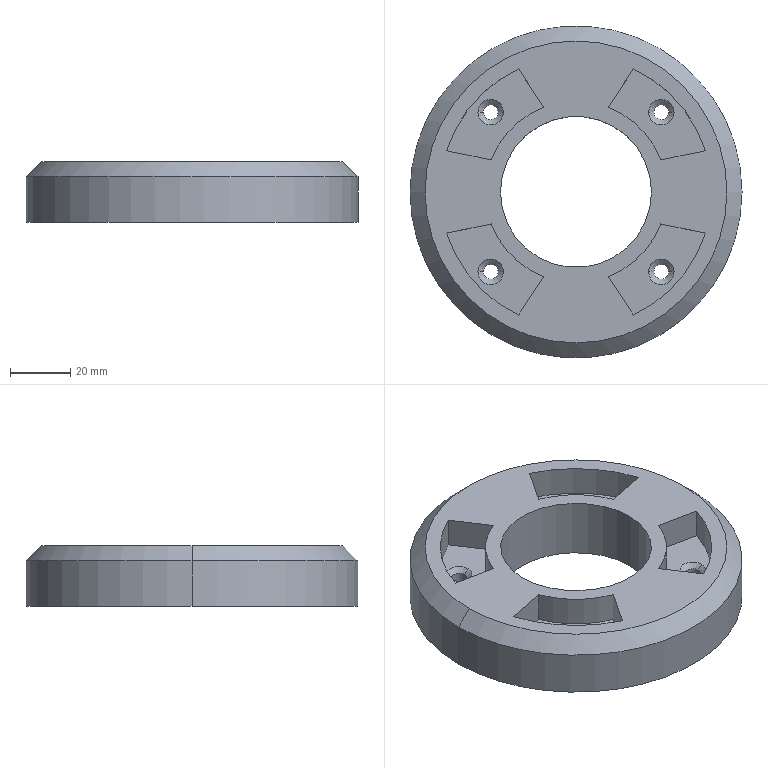Part | SolidWorks | features MirrorPattern 2, 3DProfileFeature 1, Chamfer 1, Extrusion 1, HoleWzd 1, ICE 1 | 1 solid | 44 faces | box 110 x 110 x 20 mm | volume 126964 mm3 | cylinder 20 | plane 14 | cone 10 | commonest cylinder face diameters 4.915 x8 60 x4 90 x4 50 x2 110 x2
STEP:
#1=CARTESIAN_POINT('',(25.827,-26.458,8.524));
#2=VERTEX_POINT('',#1);
#3=CARTESIAN_POINT('',(30.742,-26.458,8.524));
#4=VERTEX_POINT('',#3);
#5=CARTESIAN_POINT('',(28.284,-26.458,8.524));
#6=DIRECTION('',(0.,0.,1.));
#7=DIRECTION('',(1.,0.,0.));
#8=AXIS2_PLACEMENT_3D('',#5,#6,#7);
#9=CIRCLE('',#8,2.457);
#10=EDGE_CURVE('',#2,#4,#9,.T.);
#11=ORIENTED_EDGE('',*,*,#10,.F.);
#12=CARTESIAN_POINT('',(24.068,-26.458,10.));
#13=VERTEX_POINT('',#12);
#14=CARTESIAN_POINT('',(24.068,-26.458,10.));
#15=DIRECTION('',(-0.766,0.,0.6428));
#16=VECTOR('',#15,1000.);
#17=LINE('',#14,#16);
#18=EDGE_CURVE('',#2,#13,#17,.T.);
#19=ORIENTED_EDGE('',*,*,#18,.T.);
#20=CARTESIAN_POINT('',(32.501,-26.458,10.));
#21=VERTEX_POINT('',#20);
#22=CARTESIAN_POINT('',(28.284,-26.458,10.));
#23=DIRECTION('',(0.,0.,1.));
#24=DIRECTION('',(1.,0.,0.));
#25=AXIS2_PLACEMENT_3D('',#22,#23,#24);
#26=CIRCLE('',#25,4.216);
#27=EDGE_CURVE('',#13,#21,#26,.T.);
#28=ORIENTED_EDGE('',*,*,#27,.T.);
#29=CARTESIAN_POINT('',(32.501,-26.458,10.));
#30=DIRECTION('',(0.766,0.,0.6428));
#31=VECTOR('',#30,1000.);
#32=LINE('',#29,#31);
#33=EDGE_CURVE('',#4,#21,#32,.T.);
#34=ORIENTED_EDGE('',*,*,#33,.F.);
#35=EDGE_LOOP('',(#11,#19,#28,#34));
#36=FACE_OUTER_BOUND('',#35,.T.);
#37=CARTESIAN_POINT('',(28.284,-26.458,10.));
#38=DIRECTION('',(0.,0.,1.));
#39=DIRECTION('',(1.,0.,0.));
#40=AXIS2_PLACEMENT_3D('',#37,#38,#39);
#41=CONICAL_SURFACE('',#40,4.216,0.8727);
#42=ADVANCED_FACE('',(#36),#41,.F.);
#43=CARTESIAN_POINT('',(25.827,-26.458,0.));
#44=VERTEX_POINT('',#43);
#45=CARTESIAN_POINT('',(30.742,-26.458,0.));
#46=VERTEX_POINT('',#45);
#47=CARTESIAN_POINT('',(28.284,-26.458,0.));
#48=DIRECTION('',(0.,0.,1.));
#49=DIRECTION('',(1.,0.,0.));
#50=AXIS2_PLACEMENT_3D('',#47,#48,#49);
#51=CIRCLE('',#50,2.457);
#52=EDGE_CURVE('',#44,#46,#51,.T.);
#53=ORIENTED_EDGE('',*,*,#52,.F.);
#54=CARTESIAN_POINT('',(25.827,-26.458,10.));
#55=DIRECTION('',(0.,0.,1.));
#56=VECTOR('',#55,1000.);
#57=LINE('',#54,#56);
#58=EDGE_CURVE('',#44,#2,#57,.T.);
#59=ORIENTED_EDGE('',*,*,#58,.T.);
#60=ORIENTED_EDGE('',*,*,#10,.T.);
#61=CARTESIAN_POINT('',(30.742,-26.458,10.));
#62=DIRECTION('',(0.,0.,1.));
#63=VECTOR('',#62,1000.);
#64=LINE('',#61,#63);
#65=EDGE_CURVE('',#46,#4,#64,.T.);
#66=ORIENTED_EDGE('',*,*,#65,.F.);
#67=EDGE_LOOP('',(#53,#59,#60,#66));
#68=FACE_OUTER_BOUND('',#67,.T.);
#69=CARTESIAN_POINT('',(28.284,-26.458,10.));
#70=DIRECTION('',(0.,0.,1.));
#71=DIRECTION('',(1.,0.,0.));
#72=AXIS2_PLACEMENT_3D('',#69,#70,#71);
#73=CYLINDRICAL_SURFACE('',#72,2.457);
#74=ADVANCED_FACE('',(#68),#73,.F.);
#75=CARTESIAN_POINT('',(-30.742,-26.458,8.524));
#76=VERTEX_POINT('',#75);
#77=CARTESIAN_POINT('',(-25.827,-26.458,8.524));
#78=VERTEX_POINT('',#77);
#79=CARTESIAN_POINT('',(-28.284,-26.458,8.524));
#80=DIRECTION('',(0.,0.,1.));
#81=DIRECTION('',(1.,0.,0.));
#82=AXIS2_PLACEMENT_3D('',#79,#80,#81);
#83=CIRCLE('',#82,2.457);
#84=EDGE_CURVE('',#76,#78,#83,.T.);
#85=ORIENTED_EDGE('',*,*,#84,.F.);
#86=CARTESIAN_POINT('',(-32.501,-26.458,10.));
#87=VERTEX_POINT('',#86);
#88=CARTESIAN_POINT('',(-32.501,-26.458,10.));
#89=DIRECTION('',(-0.766,0.,0.6428));
#90=VECTOR('',#89,1000.);
#91=LINE('',#88,#90);
#92=EDGE_CURVE('',#76,#87,#91,.T.);
#93=ORIENTED_EDGE('',*,*,#92,.T.);
#94=CARTESIAN_POINT('',(-24.068,-26.458,10.));
#95=VERTEX_POINT('',#94);
#96=CARTESIAN_POINT('',(-28.284,-26.458,10.));
#97=DIRECTION('',(0.,0.,1.));
#98=DIRECTION('',(1.,0.,0.));
#99=AXIS2_PLACEMENT_3D('',#96,#97,#98);
#100=CIRCLE('',#99,4.216);
#101=EDGE_CURVE('',#87,#95,#100,.T.);
#102=ORIENTED_EDGE('',*,*,#101,.T.);
#103=CARTESIAN_POINT('',(-24.068,-26.458,10.));
#104=DIRECTION('',(0.766,0.,0.6428));
#105=VECTOR('',#104,1000.);
#106=LINE('',#103,#105);
#107=EDGE_CURVE('',#78,#95,#106,.T.);
#108=ORIENTED_EDGE('',*,*,#107,.F.);
#109=EDGE_LOOP('',(#85,#93,#102,#108));
#110=FACE_OUTER_BOUND('',#109,.T.);
#111=CARTESIAN_POINT('',(-28.284,-26.458,10.));
#112=DIRECTION('',(0.,0.,1.));
#113=DIRECTION('',(1.,0.,0.));
#114=AXIS2_PLACEMENT_3D('',#111,#112,#113);
#115=CONICAL_SURFACE('',#114,4.216,0.8727);
#116=ADVANCED_FACE('',(#110),#115,.F.);
#117=CARTESIAN_POINT('',(-30.742,-26.458,0.));
#118=VERTEX_POINT('',#117);
#119=CARTESIAN_POINT('',(-25.827,-26.458,0.));
#120=VERTEX_POINT('',#119);
#121=CARTESIAN_POINT('',(-28.284,-26.458,0.));
#122=DIRECTION('',(0.,0.,1.));
#123=DIRECTION('',(1.,0.,0.));
#124=AXIS2_PLACEMENT_3D('',#121,#122,#123);
#125=CIRCLE('',#124,2.457);
#126=EDGE_CURVE('',#118,#120,#125,.T.);
#127=ORIENTED_EDGE('',*,*,#126,.F.);
#128=CARTESIAN_POINT('',(-30.742,-26.458,10.));
#129=DIRECTION('',(0.,0.,1.));
#130=VECTOR('',#129,1000.);
#131=LINE('',#128,#130);
#132=EDGE_CURVE('',#118,#76,#131,.T.);
#133=ORIENTED_EDGE('',*,*,#132,.T.);
#134=ORIENTED_EDGE('',*,*,#84,.T.);
#135=CARTESIAN_POINT('',(-25.827,-26.458,10.));
#136=DIRECTION('',(0.,0.,1.));
#137=VECTOR('',#136,1000.);
#138=LINE('',#135,#137);
#139=EDGE_CURVE('',#120,#78,#138,.T.);
#140=ORIENTED_EDGE('',*,*,#139,.F.);
#141=EDGE_LOOP('',(#127,#133,#134,#140));
#142=FACE_OUTER_BOUND('',#141,.T.);
#143=CARTESIAN_POINT('',(-28.284,-26.458,10.));
#144=DIRECTION('',(0.,0.,1.));
#145=DIRECTION('',(1.,0.,0.));
#146=AXIS2_PLACEMENT_3D('',#143,#144,#145);
#147=CYLINDRICAL_SURFACE('',#146,2.457);
#148=ADVANCED_FACE('',(#142),#147,.F.);
#149=CARTESIAN_POINT('',(25.827,26.458,8.524));
#150=VERTEX_POINT('',#149);
#151=CARTESIAN_POINT('',(30.742,26.458,8.524));
#152=VERTEX_POINT('',#151);
#153=CARTESIAN_POINT('',(28.284,26.458,8.524));
#154=DIRECTION('',(0.,0.,1.));
#155=DIRECTION('',(1.,0.,0.));
#156=AXIS2_PLACEMENT_3D('',#153,#154,#155);
#157=CIRCLE('',#156,2.457);
#158=EDGE_CURVE('',#150,#152,#157,.T.);
#159=ORIENTED_EDGE('',*,*,#158,.F.);
#160=CARTESIAN_POINT('',(24.068,26.458,10.));
#161=VERTEX_POINT('',#160);
#162=CARTESIAN_POINT('',(24.068,26.458,10.));
#163=DIRECTION('',(-0.766,0.,0.6428));
#164=VECTOR('',#163,1000.);
#165=LINE('',#162,#164);
#166=EDGE_CURVE('',#150,#161,#165,.T.);
#167=ORIENTED_EDGE('',*,*,#166,.T.);
#168=CARTESIAN_POINT('',(32.501,26.458,10.));
#169=VERTEX_POINT('',#168);
#170=CARTESIAN_POINT('',(28.284,26.458,10.));
#171=DIRECTION('',(0.,0.,1.));
#172=DIRECTION('',(1.,0.,0.));
#173=AXIS2_PLACEMENT_3D('',#170,#171,#172);
#174=CIRCLE('',#173,4.216);
#175=EDGE_CURVE('',#161,#169,#174,.T.);
#176=ORIENTED_EDGE('',*,*,#175,.T.);
#177=CARTESIAN_POINT('',(32.501,26.458,10.));
#178=DIRECTION('',(0.766,0.,0.6428));
#179=VECTOR('',#178,1000.);
#180=LINE('',#177,#179);
#181=EDGE_CURVE('',#152,#169,#180,.T.);
#182=ORIENTED_EDGE('',*,*,#181,.F.);
#183=EDGE_LOOP('',(#159,#167,#176,#182));
#184=FACE_OUTER_BOUND('',#183,.T.);
#185=CARTESIAN_POINT('',(28.284,26.458,10.));
#186=DIRECTION('',(0.,0.,1.));
#187=DIRECTION('',(1.,0.,0.));
#188=AXIS2_PLACEMENT_3D('',#185,#186,#187);
#189=CONICAL_SURFACE('',#188,4.216,0.8727);
#190=ADVANCED_FACE('',(#184),#189,.F.);
#191=CARTESIAN_POINT('',(25.827,26.458,0.));
#192=VERTEX_POINT('',#191);
#193=CARTESIAN_POINT('',(30.742,26.458,0.));
#194=VERTEX_POINT('',#193);
#195=CARTESIAN_POINT('',(28.284,26.458,0.));
#196=DIRECTION('',(0.,0.,1.));
#197=DIRECTION('',(1.,0.,0.));
#198=AXIS2_PLACEMENT_3D('',#195,#196,#197);
#199=CIRCLE('',#198,2.457);
#200=EDGE_CURVE('',#192,#194,#199,.T.);
#201=ORIENTED_EDGE('',*,*,#200,.F.);
#202=CARTESIAN_POINT('',(25.827,26.458,10.));
#203=DIRECTION('',(0.,0.,1.));
#204=VECTOR('',#203,1000.);
#205=LINE('',#202,#204);
#206=EDGE_CURVE('',#192,#150,#205,.T.);
#207=ORIENTED_EDGE('',*,*,#206,.T.);
#208=ORIENTED_EDGE('',*,*,#158,.T.);
#209=CARTESIAN_POINT('',(30.742,26.458,10.));
#210=DIRECTION('',(0.,0.,1.));
#211=VECTOR('',#210,1000.);
#212=LINE('',#209,#211);
#213=EDGE_CURVE('',#194,#152,#212,.T.);
#214=ORIENTED_EDGE('',*,*,#213,.F.);
#215=EDGE_LOOP('',(#201,#207,#208,#214));
#216=FACE_OUTER_BOUND('',#215,.T.);
#217=CARTESIAN_POINT('',(28.284,26.458,10.));
#218=DIRECTION('',(0.,0.,1.));
#219=DIRECTION('',(1.,0.,0.));
#220=AXIS2_PLACEMENT_3D('',#217,#218,#219);
#221=CYLINDRICAL_SURFACE('',#220,2.457);
#222=ADVANCED_FACE('',(#216),#221,.F.);
#223=CARTESIAN_POINT('',(-30.742,26.458,8.524));
#224=VERTEX_POINT('',#223);
#225=CARTESIAN_POINT('',(-25.827,26.458,8.524));
#226=VERTEX_POINT('',#225);
#227=CARTESIAN_POINT('',(-28.284,26.458,8.524));
#228=DIRECTION('',(0.,0.,1.));
#229=DIRECTION('',(1.,0.,0.));
#230=AXIS2_PLACEMENT_3D('',#227,#228,#229);
#231=CIRCLE('',#230,2.457);
#232=EDGE_CURVE('',#224,#226,#231,.T.);
#233=ORIENTED_EDGE('',*,*,#232,.F.);
#234=CARTESIAN_POINT('',(-32.501,26.458,10.));
#235=VERTEX_POINT('',#234);
#236=CARTESIAN_POINT('',(-32.501,26.458,10.));
#237=DIRECTION('',(-0.766,0.,0.6428));
#238=VECTOR('',#237,1000.);
#239=LINE('',#236,#238);
#240=EDGE_CURVE('',#224,#235,#239,.T.);
#241=ORIENTED_EDGE('',*,*,#240,.T.);
#242=CARTESIAN_POINT('',(-24.068,26.458,10.));
#243=VERTEX_POINT('',#242);
#244=CARTESIAN_POINT('',(-28.284,26.458,10.));
#245=DIRECTION('',(0.,0.,1.));
#246=DIRECTION('',(1.,0.,0.));
#247=AXIS2_PLACEMENT_3D('',#244,#245,#246);
#248=CIRCLE('',#247,4.216);
#249=EDGE_CURVE('',#235,#243,#248,.T.);
#250=ORIENTED_EDGE('',*,*,#249,.T.);
#251=CARTESIAN_POINT('',(-24.068,26.458,10.));
#252=DIRECTION('',(0.766,0.,0.6428));
#253=VECTOR('',#252,1000.);
#254=LINE('',#251,#253);
#255=EDGE_CURVE('',#226,#243,#254,.T.);
#256=ORIENTED_EDGE('',*,*,#255,.F.);
#257=EDGE_LOOP('',(#233,#241,#250,#256));
#258=FACE_OUTER_BOUND('',#257,.T.);
#259=CARTESIAN_POINT('',(-28.284,26.458,10.));
#260=DIRECTION('',(0.,0.,1.));
#261=DIRECTION('',(1.,0.,0.));
#262=AXIS2_PLACEMENT_3D('',#259,#260,#261);
#263=CONICAL_SURFACE('',#262,4.216,0.8727);
#264=ADVANCED_FACE('',(#258),#263,.F.);
#265=CARTESIAN_POINT('',(-30.742,26.458,0.));
#266=VERTEX_POINT('',#265);
#267=CARTESIAN_POINT('',(-25.827,26.458,0.));
#268=VERTEX_POINT('',#267);
#269=CARTESIAN_POINT('',(-28.284,26.458,0.));
#270=DIRECTION('',(0.,0.,1.));
#271=DIRECTION('',(1.,0.,0.));
#272=AXIS2_PLACEMENT_3D('',#269,#270,#271);
#273=CIRCLE('',#272,2.457);
#274=EDGE_CURVE('',#266,#268,#273,.T.);
#275=ORIENTED_EDGE('',*,*,#274,.F.);
#276=CARTESIAN_POINT('',(-30.742,26.458,10.));
#277=DIRECTION('',(0.,0.,1.));
#278=VECTOR('',#277,1000.);
#279=LINE('',#276,#278);
#280=EDGE_CURVE('',#266,#224,#279,.T.);
#281=ORIENTED_EDGE('',*,*,#280,.T.);
#282=ORIENTED_EDGE('',*,*,#232,.T.);
#283=CARTESIAN_POINT('',(-25.827,26.458,10.));
#284=DIRECTION('',(0.,0.,1.));
#285=VECTOR('',#284,1000.);
#286=LINE('',#283,#285);
#287=EDGE_CURVE('',#268,#226,#286,.T.);
#288=ORIENTED_EDGE('',*,*,#287,.F.);
#289=EDGE_LOOP('',(#275,#281,#282,#288));
#290=FACE_OUTER_BOUND('',#289,.T.);
#291=CARTESIAN_POINT('',(-28.284,26.458,10.));
#292=DIRECTION('',(0.,0.,1.));
#293=DIRECTION('',(1.,0.,0.));
#294=AXIS2_PLACEMENT_3D('',#291,#292,#293);
#295=CYLINDRICAL_SURFACE('',#294,2.457);
#296=ADVANCED_FACE('',(#290),#295,.F.);
#297=CARTESIAN_POINT('',(50.,0.,20.));
#298=VERTEX_POINT('',#297);
#299=CARTESIAN_POINT('',(-50.,0.,20.));
#300=VERTEX_POINT('',#299);
#301=CARTESIAN_POINT('',(0.,0.,20.));
#302=DIRECTION('',(0.,0.,1.));
#303=DIRECTION('',(1.,0.,0.));
#304=AXIS2_PLACEMENT_3D('',#301,#302,#303);
#305=CIRCLE('',#304,50.);
#306=EDGE_CURVE('',#298,#300,#305,.T.);
#307=ORIENTED_EDGE('',*,*,#306,.F.);
#308=CARTESIAN_POINT('',(55.,0.,15.));
#309=VERTEX_POINT('',#308);
#310=CARTESIAN_POINT('',(50.,0.,20.));
#311=DIRECTION('',(0.7071,0.,-0.7071));
#312=VECTOR('',#311,1000.);
#313=LINE('',#310,#312);
#314=EDGE_CURVE('',#298,#309,#313,.T.);
#315=ORIENTED_EDGE('',*,*,#314,.T.);
#316=CARTESIAN_POINT('',(-55.,0.,15.));
#317=VERTEX_POINT('',#316);
#318=CARTESIAN_POINT('',(0.,0.,15.));
#319=DIRECTION('',(0.,0.,-1.));
#320=DIRECTION('',(1.,0.,0.));
#321=AXIS2_PLACEMENT_3D('',#318,#319,#320);
#322=CIRCLE('',#321,55.);
#323=EDGE_CURVE('',#317,#309,#322,.T.);
#324=ORIENTED_EDGE('',*,*,#323,.F.);
#325=CARTESIAN_POINT('',(-50.,0.,20.));
#326=DIRECTION('',(-0.7071,0.,-0.7071));
#327=VECTOR('',#326,1000.);
#328=LINE('',#325,#327);
#329=EDGE_CURVE('',#300,#317,#328,.T.);
#330=ORIENTED_EDGE('',*,*,#329,.F.);
#331=EDGE_LOOP('',(#307,#315,#324,#330));
#332=FACE_OUTER_BOUND('',#331,.T.);
#333=CARTESIAN_POINT('',(0.,0.,20.));
#334=DIRECTION('',(0.,0.,-1.));
#335=DIRECTION('',(-1.,0.,0.));
#336=AXIS2_PLACEMENT_3D('',#333,#334,#335);
#337=CONICAL_SURFACE('',#336,50.,0.7854);
#338=ADVANCED_FACE('',(#332),#337,.T.);
#339=CARTESIAN_POINT('',(-25.,0.,20.));
#340=VERTEX_POINT('',#339);
#341=CARTESIAN_POINT('',(25.,0.,20.));
#342=VERTEX_POINT('',#341);
#343=CARTESIAN_POINT('',(0.,0.,20.));
#344=DIRECTION('',(0.,0.,1.));
#345=DIRECTION('',(1.,0.,0.));
#346=AXIS2_PLACEMENT_3D('',#343,#344,#345);
#347=CIRCLE('',#346,25.);
#348=EDGE_CURVE('',#340,#342,#347,.T.);
#349=ORIENTED_EDGE('',*,*,#348,.T.);
#350=CARTESIAN_POINT('',(25.,0.,0.));
#351=VERTEX_POINT('',#350);
#352=CARTESIAN_POINT('',(25.,0.,20.));
#353=DIRECTION('',(0.,0.,-1.));
#354=VECTOR('',#353,1000.);
#355=LINE('',#352,#354);
#356=EDGE_CURVE('',#342,#351,#355,.T.);
#357=ORIENTED_EDGE('',*,*,#356,.T.);
#358=CARTESIAN_POINT('',(-25.,0.,0.));
#359=VERTEX_POINT('',#358);
#360=CARTESIAN_POINT('',(0.,0.,0.));
#361=DIRECTION('',(0.,0.,1.));
#362=DIRECTION('',(1.,0.,0.));
#363=AXIS2_PLACEMENT_3D('',#360,#361,#362);
#364=CIRCLE('',#363,25.);
#365=EDGE_CURVE('',#359,#351,#364,.T.);
#366=ORIENTED_EDGE('',*,*,#365,.F.);
#367=CARTESIAN_POINT('',(-25.,0.,20.));
#368=DIRECTION('',(0.,0.,-1.));
#369=VECTOR('',#368,1000.);
#370=LINE('',#367,#369);
#371=EDGE_CURVE('',#340,#359,#370,.T.);
#372=ORIENTED_EDGE('',*,*,#371,.F.);
#373=EDGE_LOOP('',(#349,#357,#366,#372));
#374=FACE_OUTER_BOUND('',#373,.T.);
#375=CARTESIAN_POINT('',(0.,0.,20.));
#376=DIRECTION('',(0.,0.,-1.));
#377=DIRECTION('',(-1.,0.,0.));
#378=AXIS2_PLACEMENT_3D('',#375,#376,#377);
#379=CYLINDRICAL_SURFACE('',#378,25.);
#380=ADVANCED_FACE('',(#374),#379,.F.);
#381=ORIENTED_EDGE('',*,*,#323,.T.);
#382=CARTESIAN_POINT('',(55.,0.,0.));
#383=VERTEX_POINT('',#382);
#384=CARTESIAN_POINT('',(55.,0.,20.));
#385=DIRECTION('',(0.,0.,-1.));
#386=VECTOR('',#385,1000.);
#387=LINE('',#384,#386);
#388=EDGE_CURVE('',#309,#383,#387,.T.);
#389=ORIENTED_EDGE('',*,*,#388,.T.);
#390=CARTESIAN_POINT('',(-55.,0.,0.));
#391=VERTEX_POINT('',#390);
#392=CARTESIAN_POINT('',(0.,0.,0.));
#393=DIRECTION('',(0.,0.,1.));
#394=DIRECTION('',(1.,0.,0.));
#395=AXIS2_PLACEMENT_3D('',#392,#393,#394);
#396=CIRCLE('',#395,55.);
#397=EDGE_CURVE('',#383,#391,#396,.T.);
#398=ORIENTED_EDGE('',*,*,#397,.T.);
#399=CARTESIAN_POINT('',(-55.,0.,20.));
#400=DIRECTION('',(0.,0.,-1.));
#401=VECTOR('',#400,1000.);
#402=LINE('',#399,#401);
#403=EDGE_CURVE('',#317,#391,#402,.T.);
#404=ORIENTED_EDGE('',*,*,#403,.F.);
#405=EDGE_LOOP('',(#381,#389,#398,#404));
#406=FACE_OUTER_BOUND('',#405,.T.);
#407=CARTESIAN_POINT('',(0.,0.,20.));
#408=DIRECTION('',(0.,0.,-1.));
#409=DIRECTION('',(-1.,0.,0.));
#410=AXIS2_PLACEMENT_3D('',#407,#408,#409);
#411=CYLINDRICAL_SURFACE('',#410,55.);
#412=ADVANCED_FACE('',(#406),#411,.T.);
#413=CARTESIAN_POINT('',(0.,0.,20.));
#414=DIRECTION('',(0.,0.,1.));
#415=DIRECTION('',(1.,0.,0.));
#416=AXIS2_PLACEMENT_3D('',#413,#414,#415);
#417=CIRCLE('',#416,50.);
#418=EDGE_CURVE('',#300,#298,#417,.T.);
#419=ORIENTED_EDGE('',*,*,#418,.T.);
#420=ORIENTED_EDGE('',*,*,#306,.T.);
#421=EDGE_LOOP('',(#419,#420));
#422=FACE_OUTER_BOUND('',#421,.T.);
#423=CARTESIAN_POINT('',(-10.612,-28.06,20.));
#424=VERTEX_POINT('',#423);
#425=CARTESIAN_POINT('',(-28.06,-10.612,20.));
#426=VERTEX_POINT('',#425);
#427=CARTESIAN_POINT('',(0.,0.,20.));
#428=DIRECTION('',(0.,0.,-1.));
#429=DIRECTION('',(-1.,0.,0.));
#430=AXIS2_PLACEMENT_3D('',#427,#428,#429);
#431=CIRCLE('',#430,30.);
#432=EDGE_CURVE('',#424,#426,#431,.T.);
#433=ORIENTED_EDGE('',*,*,#432,.F.);
#434=CARTESIAN_POINT('',(-19.017,-40.784,20.));
#435=VERTEX_POINT('',#434);
#436=CARTESIAN_POINT('',(-10.612,-28.06,20.));
#437=DIRECTION('',(0.5512,0.8344,0.));
#438=VECTOR('',#437,1000.);
#439=LINE('',#436,#438);
#440=EDGE_CURVE('',#435,#424,#439,.T.);
#441=ORIENTED_EDGE('',*,*,#440,.F.);
#442=CARTESIAN_POINT('',(-42.882,-13.642,20.));
#443=VERTEX_POINT('',#442);
#444=CARTESIAN_POINT('',(0.,0.,20.));
#445=DIRECTION('',(0.,0.,1.));
#446=DIRECTION('',(-1.,0.,0.));
#447=AXIS2_PLACEMENT_3D('',#444,#445,#446);
#448=CIRCLE('',#447,45.);
#449=EDGE_CURVE('',#443,#435,#448,.T.);
#450=ORIENTED_EDGE('',*,*,#449,.F.);
#451=CARTESIAN_POINT('',(-28.06,-10.612,20.));
#452=DIRECTION('',(-0.9797,-0.2003,0.));
#453=VECTOR('',#452,1000.);
#454=LINE('',#451,#453);
#455=EDGE_CURVE('',#426,#443,#454,.T.);
#456=ORIENTED_EDGE('',*,*,#455,.F.);
#457=EDGE_LOOP('',(#433,#441,#450,#456));
#458=FACE_BOUND('',#457,.T.);
#459=CARTESIAN_POINT('',(19.017,-40.784,20.));
#460=VERTEX_POINT('',#459);
#461=CARTESIAN_POINT('',(42.882,-13.642,20.));
#462=VERTEX_POINT('',#461);
#463=CARTESIAN_POINT('',(0.,0.,20.));
#464=DIRECTION('',(0.,0.,1.));
#465=DIRECTION('',(1.,0.,0.));
#466=AXIS2_PLACEMENT_3D('',#463,#464,#465);
#467=CIRCLE('',#466,45.);
#468=EDGE_CURVE('',#460,#462,#467,.T.);
#469=ORIENTED_EDGE('',*,*,#468,.F.);
#470=CARTESIAN_POINT('',(10.612,-28.06,20.));
#471=VERTEX_POINT('',#470);
#472=CARTESIAN_POINT('',(10.612,-28.06,20.));
#473=DIRECTION('',(0.5512,-0.8344,0.));
#474=VECTOR('',#473,1000.);
#475=LINE('',#472,#474);
#476=EDGE_CURVE('',#471,#460,#475,.T.);
#477=ORIENTED_EDGE('',*,*,#476,.F.);
#478=CARTESIAN_POINT('',(28.06,-10.612,20.));
#479=VERTEX_POINT('',#478);
#480=CARTESIAN_POINT('',(0.,0.,20.));
#481=DIRECTION('',(0.,0.,-1.));
#482=DIRECTION('',(1.,0.,0.));
#483=AXIS2_PLACEMENT_3D('',#480,#481,#482);
#484=CIRCLE('',#483,30.);
#485=EDGE_CURVE('',#479,#471,#484,.T.);
#486=ORIENTED_EDGE('',*,*,#485,.F.);
#487=CARTESIAN_POINT('',(28.06,-10.612,20.));
#488=DIRECTION('',(-0.9797,0.2003,0.));
#489=VECTOR('',#488,1000.);
#490=LINE('',#487,#489);
#491=EDGE_CURVE('',#462,#479,#490,.T.);
#492=ORIENTED_EDGE('',*,*,#491,.F.);
#493=EDGE_LOOP('',(#469,#477,#486,#492));
#494=FACE_BOUND('',#493,.T.);
#495=CARTESIAN_POINT('',(10.612,28.06,20.));
#496=VERTEX_POINT('',#495);
#497=CARTESIAN_POINT('',(28.06,10.612,20.));
#498=VERTEX_POINT('',#497);
#499=CARTESIAN_POINT('',(0.,0.,20.));
#500=DIRECTION('',(0.,0.,-1.));
#501=DIRECTION('',(-1.,0.,0.));
#502=AXIS2_PLACEMENT_3D('',#499,#500,#501);
#503=CIRCLE('',#502,30.);
#504=EDGE_CURVE('',#496,#498,#503,.T.);
#505=ORIENTED_EDGE('',*,*,#504,.F.);
#506=CARTESIAN_POINT('',(19.017,40.784,20.));
#507=VERTEX_POINT('',#506);
#508=CARTESIAN_POINT('',(10.612,28.06,20.));
#509=DIRECTION('',(-0.5512,-0.8344,0.));
#510=VECTOR('',#509,1000.);
#511=LINE('',#508,#510);
#512=EDGE_CURVE('',#507,#496,#511,.T.);
#513=ORIENTED_EDGE('',*,*,#512,.F.);
#514=CARTESIAN_POINT('',(42.882,13.642,20.));
#515=VERTEX_POINT('',#514);
#516=CARTESIAN_POINT('',(0.,0.,20.));
#517=DIRECTION('',(0.,0.,1.));
#518=DIRECTION('',(-1.,0.,0.));
#519=AXIS2_PLACEMENT_3D('',#516,#517,#518);
#520=CIRCLE('',#519,45.);
#521=EDGE_CURVE('',#515,#507,#520,.T.);
#522=ORIENTED_EDGE('',*,*,#521,.F.);
#523=CARTESIAN_POINT('',(28.06,10.612,20.));
#524=DIRECTION('',(0.9797,0.2003,0.));
#525=VECTOR('',#524,1000.);
#526=LINE('',#523,#525);
#527=EDGE_CURVE('',#498,#515,#526,.T.);
#528=ORIENTED_EDGE('',*,*,#527,.F.);
#529=EDGE_LOOP('',(#505,#513,#522,#528));
#530=FACE_BOUND('',#529,.T.);
#531=CARTESIAN_POINT('',(-28.06,10.612,20.));
#532=VERTEX_POINT('',#531);
#533=CARTESIAN_POINT('',(-10.612,28.06,20.));
#534=VERTEX_POINT('',#533);
#535=CARTESIAN_POINT('',(0.,0.,20.));
#536=DIRECTION('',(0.,0.,-1.));
#537=DIRECTION('',(1.,0.,0.));
#538=AXIS2_PLACEMENT_3D('',#535,#536,#537);
#539=CIRCLE('',#538,30.);
#540=EDGE_CURVE('',#532,#534,#539,.T.);
#541=ORIENTED_EDGE('',*,*,#540,.F.);
#542=CARTESIAN_POINT('',(-42.882,13.642,20.));
#543=VERTEX_POINT('',#542);
#544=CARTESIAN_POINT('',(-28.06,10.612,20.));
#545=DIRECTION('',(0.9797,-0.2003,0.));
#546=VECTOR('',#545,1000.);
#547=LINE('',#544,#546);
#548=EDGE_CURVE('',#543,#532,#547,.T.);
#549=ORIENTED_EDGE('',*,*,#548,.F.);
#550=CARTESIAN_POINT('',(-19.017,40.784,20.));
#551=VERTEX_POINT('',#550);
#552=CARTESIAN_POINT('',(0.,0.,20.));
#553=DIRECTION('',(0.,0.,1.));
#554=DIRECTION('',(1.,0.,0.));
#555=AXIS2_PLACEMENT_3D('',#552,#553,#554);
#556=CIRCLE('',#555,45.);
#557=EDGE_CURVE('',#551,#543,#556,.T.);
#558=ORIENTED_EDGE('',*,*,#557,.F.);
#559=CARTESIAN_POINT('',(-10.612,28.06,20.));
#560=DIRECTION('',(-0.5512,0.8344,0.));
#561=VECTOR('',#560,1000.);
#562=LINE('',#559,#561);
#563=EDGE_CURVE('',#534,#551,#562,.T.);
#564=ORIENTED_EDGE('',*,*,#563,.F.);
#565=EDGE_LOOP('',(#541,#549,#558,#564));
#566=FACE_BOUND('',#565,.T.);
#567=ORIENTED_EDGE('',*,*,#348,.F.);
#568=CARTESIAN_POINT('',(0.,0.,20.));
#569=DIRECTION('',(0.,0.,1.));
#570=DIRECTION('',(1.,0.,0.));
#571=AXIS2_PLACEMENT_3D('',#568,#569,#570);
#572=CIRCLE('',#571,25.);
#573=EDGE_CURVE('',#342,#340,#572,.T.);
#574=ORIENTED_EDGE('',*,*,#573,.F.);
#575=EDGE_LOOP('',(#567,#574));
#576=FACE_BOUND('',#575,.T.);
#577=CARTESIAN_POINT('',(0.,0.,20.));
#578=DIRECTION('',(0.,0.,1.));
#579=DIRECTION('',(1.,0.,0.));
#580=AXIS2_PLACEMENT_3D('',#577,#578,#579);
#581=PLANE('',#580);
#582=ADVANCED_FACE('',(#422,#458,#494,#530,#566,#576),#581,.T.);
#583=CARTESIAN_POINT('',(28.284,-26.458,0.));
#584=DIRECTION('',(0.,0.,1.));
#585=DIRECTION('',(1.,0.,0.));
#586=AXIS2_PLACEMENT_3D('',#583,#584,#585);
#587=CIRCLE('',#586,2.457);
#588=EDGE_CURVE('',#46,#44,#587,.T.);
#589=ORIENTED_EDGE('',*,*,#588,.T.);
#590=ORIENTED_EDGE('',*,*,#52,.T.);
#591=EDGE_LOOP('',(#589,#590));
#592=FACE_BOUND('',#591,.T.);
#593=CARTESIAN_POINT('',(-28.284,-26.458,0.));
#594=DIRECTION('',(0.,0.,1.));
#595=DIRECTION('',(1.,0.,0.));
#596=AXIS2_PLACEMENT_3D('',#593,#594,#595);
#597=CIRCLE('',#596,2.457);
#598=EDGE_CURVE('',#120,#118,#597,.T.);
#599=ORIENTED_EDGE('',*,*,#598,.T.);
#600=ORIENTED_EDGE('',*,*,#126,.T.);
#601=EDGE_LOOP('',(#599,#600));
#602=FACE_BOUND('',#601,.T.);
#603=CARTESIAN_POINT('',(28.284,26.458,0.));
#604=DIRECTION('',(0.,0.,1.));
#605=DIRECTION('',(1.,0.,0.));
#606=AXIS2_PLACEMENT_3D('',#603,#604,#605);
#607=CIRCLE('',#606,2.457);
#608=EDGE_CURVE('',#194,#192,#607,.T.);
#609=ORIENTED_EDGE('',*,*,#608,.T.);
#610=ORIENTED_EDGE('',*,*,#200,.T.);
#611=EDGE_LOOP('',(#609,#610));
#612=FACE_BOUND('',#611,.T.);
#613=CARTESIAN_POINT('',(-28.284,26.458,0.));
#614=DIRECTION('',(0.,0.,1.));
#615=DIRECTION('',(1.,0.,0.));
#616=AXIS2_PLACEMENT_3D('',#613,#614,#615);
#617=CIRCLE('',#616,2.457);
#618=EDGE_CURVE('',#268,#266,#617,.T.);
#619=ORIENTED_EDGE('',*,*,#618,.T.);
#620=ORIENTED_EDGE('',*,*,#274,.T.);
#621=EDGE_LOOP('',(#619,#620));
#622=FACE_BOUND('',#621,.T.);
#623=CARTESIAN_POINT('',(0.,0.,0.));
#624=DIRECTION('',(0.,0.,1.));
#625=DIRECTION('',(1.,0.,0.));
#626=AXIS2_PLACEMENT_3D('',#623,#624,#625);
#627=CIRCLE('',#626,55.);
#628=EDGE_CURVE('',#391,#383,#627,.T.);
#629=ORIENTED_EDGE('',*,*,#628,.F.);
#630=ORIENTED_EDGE('',*,*,#397,.F.);
#631=EDGE_LOOP('',(#629,#630));
#632=FACE_OUTER_BOUND('',#631,.T.);
#633=ORIENTED_EDGE('',*,*,#365,.T.);
#634=CARTESIAN_POINT('',(0.,0.,0.));
#635=DIRECTION('',(0.,0.,1.));
#636=DIRECTION('',(1.,0.,0.));
#637=AXIS2_PLACEMENT_3D('',#634,#635,#636);
#638=CIRCLE('',#637,25.);
#639=EDGE_CURVE('',#351,#359,#638,.T.);
#640=ORIENTED_EDGE('',*,*,#639,.T.);
#641=EDGE_LOOP('',(#633,#640));
#642=FACE_BOUND('',#641,.T.);
#643=CARTESIAN_POINT('',(0.,0.,0.));
#644=DIRECTION('',(0.,0.,1.));
#645=DIRECTION('',(1.,0.,0.));
#646=AXIS2_PLACEMENT_3D('',#643,#644,#645);
#647=PLANE('',#646);
#648=ADVANCED_FACE('',(#592,#602,#612,#622,#632,#642),#647,.F.);
#649=ORIENTED_EDGE('',*,*,#388,.F.);
#650=CARTESIAN_POINT('',(0.,0.,15.));
#651=DIRECTION('',(0.,0.,-1.));
#652=DIRECTION('',(1.,0.,0.));
#653=AXIS2_PLACEMENT_3D('',#650,#651,#652);
#654=CIRCLE('',#653,55.);
#655=EDGE_CURVE('',#309,#317,#654,.T.);
#656=ORIENTED_EDGE('',*,*,#655,.T.);
#657=ORIENTED_EDGE('',*,*,#403,.T.);
#658=ORIENTED_EDGE('',*,*,#628,.T.);
#659=EDGE_LOOP('',(#649,#656,#657,#658));
#660=FACE_OUTER_BOUND('',#659,.T.);
#661=CARTESIAN_POINT('',(0.,0.,20.));
#662=DIRECTION('',(0.,0.,-1.));
#663=DIRECTION('',(-1.,0.,0.));
#664=AXIS2_PLACEMENT_3D('',#661,#662,#663);
#665=CYLINDRICAL_SURFACE('',#664,55.);
#666=ADVANCED_FACE('',(#660),#665,.T.);
#667=ORIENTED_EDGE('',*,*,#356,.F.);
#668=ORIENTED_EDGE('',*,*,#573,.T.);
#669=ORIENTED_EDGE('',*,*,#371,.T.);
#670=ORIENTED_EDGE('',*,*,#639,.F.);
#671=EDGE_LOOP('',(#667,#668,#669,#670));
#672=FACE_OUTER_BOUND('',#671,.T.);
#673=CARTESIAN_POINT('',(0.,0.,20.));
#674=DIRECTION('',(0.,0.,-1.));
#675=DIRECTION('',(-1.,0.,0.));
#676=AXIS2_PLACEMENT_3D('',#673,#674,#675);
#677=CYLINDRICAL_SURFACE('',#676,25.);
#678=ADVANCED_FACE('',(#672),#677,.F.);
#679=ORIENTED_EDGE('',*,*,#540,.T.);
#680=CARTESIAN_POINT('',(-10.612,28.06,10.));
#681=VERTEX_POINT('',#680);
#682=CARTESIAN_POINT('',(-10.612,28.06,10.));
#683=DIRECTION('',(0.,0.,1.));
#684=VECTOR('',#683,1000.);
#685=LINE('',#682,#684);
#686=EDGE_CURVE('',#681,#534,#685,.T.);
#687=ORIENTED_EDGE('',*,*,#686,.F.);
#688=CARTESIAN_POINT('',(-28.06,10.612,10.));
#689=VERTEX_POINT('',#688);
#690=CARTESIAN_POINT('',(0.,0.,10.));
#691=DIRECTION('',(0.,0.,-1.));
#692=DIRECTION('',(1.,0.,0.));
#693=AXIS2_PLACEMENT_3D('',#690,#691,#692);
#694=CIRCLE('',#693,30.);
#695=EDGE_CURVE('',#689,#681,#694,.T.);
#696=ORIENTED_EDGE('',*,*,#695,.F.);
#697=CARTESIAN_POINT('',(-28.06,10.612,10.));
#698=DIRECTION('',(0.,0.,1.));
#699=VECTOR('',#698,1000.);
#700=LINE('',#697,#699);
#701=EDGE_CURVE('',#689,#532,#700,.T.);
#702=ORIENTED_EDGE('',*,*,#701,.T.);
#703=EDGE_LOOP('',(#679,#687,#696,#702));
#704=FACE_OUTER_BOUND('',#703,.T.);
#705=CARTESIAN_POINT('',(0.,0.,10.));
#706=DIRECTION('',(0.,0.,1.));
#707=DIRECTION('',(1.,0.,0.));
#708=AXIS2_PLACEMENT_3D('',#705,#706,#707);
#709=CYLINDRICAL_SURFACE('',#708,30.);
#710=ADVANCED_FACE('',(#704),#709,.T.);
#711=ORIENTED_EDGE('',*,*,#548,.T.);
#712=ORIENTED_EDGE('',*,*,#701,.F.);
#713=CARTESIAN_POINT('',(-42.882,13.642,10.));
#714=VERTEX_POINT('',#713);
#715=CARTESIAN_POINT('',(-28.06,10.612,10.));
#716=DIRECTION('',(0.9797,-0.2003,0.));
#717=VECTOR('',#716,1000.);
#718=LINE('',#715,#717);
#719=EDGE_CURVE('',#714,#689,#718,.T.);
#720=ORIENTED_EDGE('',*,*,#719,.F.);
#721=CARTESIAN_POINT('',(-42.882,13.642,10.));
#722=DIRECTION('',(0.,0.,1.));
#723=VECTOR('',#722,1000.);
#724=LINE('',#721,#723);
#725=EDGE_CURVE('',#714,#543,#724,.T.);
#726=ORIENTED_EDGE('',*,*,#725,.T.);
#727=EDGE_LOOP('',(#711,#712,#720,#726));
#728=FACE_OUTER_BOUND('',#727,.T.);
#729=CARTESIAN_POINT('',(-28.06,10.612,10.));
#730=DIRECTION('',(-0.2003,-0.9797,0.));
#731=DIRECTION('',(0.9797,-0.2003,0.));
#732=AXIS2_PLACEMENT_3D('',#729,#730,#731);
#733=PLANE('',#732);
#734=ADVANCED_FACE('',(#728),#733,.F.);
#735=ORIENTED_EDGE('',*,*,#557,.T.);
#736=ORIENTED_EDGE('',*,*,#725,.F.);
#737=CARTESIAN_POINT('',(-19.017,40.784,10.));
#738=VERTEX_POINT('',#737);
#739=CARTESIAN_POINT('',(0.,0.,10.));
#740=DIRECTION('',(0.,0.,1.));
#741=DIRECTION('',(1.,0.,0.));
#742=AXIS2_PLACEMENT_3D('',#739,#740,#741);
#743=CIRCLE('',#742,45.);
#744=EDGE_CURVE('',#738,#714,#743,.T.);
#745=ORIENTED_EDGE('',*,*,#744,.F.);
#746=CARTESIAN_POINT('',(-19.017,40.784,10.));
#747=DIRECTION('',(0.,0.,1.));
#748=VECTOR('',#747,1000.);
#749=LINE('',#746,#748);
#750=EDGE_CURVE('',#738,#551,#749,.T.);
#751=ORIENTED_EDGE('',*,*,#750,.T.);
#752=EDGE_LOOP('',(#735,#736,#745,#751));
#753=FACE_OUTER_BOUND('',#752,.T.);
#754=CARTESIAN_POINT('',(0.,0.,10.));
#755=DIRECTION('',(0.,0.,1.));
#756=DIRECTION('',(1.,0.,0.));
#757=AXIS2_PLACEMENT_3D('',#754,#755,#756);
#758=CYLINDRICAL_SURFACE('',#757,45.);
#759=ADVANCED_FACE('',(#753),#758,.F.);
#760=ORIENTED_EDGE('',*,*,#563,.T.);
#761=ORIENTED_EDGE('',*,*,#750,.F.);
#762=CARTESIAN_POINT('',(-10.612,28.06,10.));
#763=DIRECTION('',(-0.5512,0.8344,0.));
#764=VECTOR('',#763,1000.);
#765=LINE('',#762,#764);
#766=EDGE_CURVE('',#681,#738,#765,.T.);
#767=ORIENTED_EDGE('',*,*,#766,.F.);
#768=ORIENTED_EDGE('',*,*,#686,.T.);
#769=EDGE_LOOP('',(#760,#761,#767,#768));
#770=FACE_OUTER_BOUND('',#769,.T.);
#771=CARTESIAN_POINT('',(-10.612,28.06,10.));
#772=DIRECTION('',(0.8344,0.5512,0.));
#773=DIRECTION('',(-0.5512,0.8344,0.));
#774=AXIS2_PLACEMENT_3D('',#771,#772,#773);
#775=PLANE('',#774);
#776=ADVANCED_FACE('',(#770),#775,.F.);
#777=CARTESIAN_POINT('',(-28.284,26.458,10.));
#778=DIRECTION('',(0.,0.,1.));
#779=DIRECTION('',(1.,0.,0.));
#780=AXIS2_PLACEMENT_3D('',#777,#778,#779);
#781=CIRCLE('',#780,4.216);
#782=EDGE_CURVE('',#243,#235,#781,.T.);
#783=ORIENTED_EDGE('',*,*,#782,.F.);
#784=ORIENTED_EDGE('',*,*,#249,.F.);
#785=EDGE_LOOP('',(#783,#784));
#786=FACE_BOUND('',#785,.T.);
#787=ORIENTED_EDGE('',*,*,#695,.T.);
#788=ORIENTED_EDGE('',*,*,#766,.T.);
#789=ORIENTED_EDGE('',*,*,#744,.T.);
#790=ORIENTED_EDGE('',*,*,#719,.T.);
#791=EDGE_LOOP('',(#787,#788,#789,#790));
#792=FACE_OUTER_BOUND('',#791,.T.);
#793=CARTESIAN_POINT('',(0.,0.,10.));
#794=DIRECTION('',(0.,0.,1.));
#795=DIRECTION('',(1.,0.,0.));
#796=AXIS2_PLACEMENT_3D('',#793,#794,#795);
#797=PLANE('',#796);
#798=ADVANCED_FACE('',(#786,#792),#797,.T.);
#799=ORIENTED_EDGE('',*,*,#504,.T.);
#800=CARTESIAN_POINT('',(28.06,10.612,10.));
#801=VERTEX_POINT('',#800);
#802=CARTESIAN_POINT('',(28.06,10.612,10.));
#803=DIRECTION('',(0.,0.,1.));
#804=VECTOR('',#803,1000.);
#805=LINE('',#802,#804);
#806=EDGE_CURVE('',#801,#498,#805,.T.);
#807=ORIENTED_EDGE('',*,*,#806,.F.);
#808=CARTESIAN_POINT('',(10.612,28.06,10.));
#809=VERTEX_POINT('',#808);
#810=CARTESIAN_POINT('',(0.,0.,10.));
#811=DIRECTION('',(0.,0.,-1.));
#812=DIRECTION('',(-1.,0.,0.));
#813=AXIS2_PLACEMENT_3D('',#810,#811,#812);
#814=CIRCLE('',#813,30.);
#815=EDGE_CURVE('',#809,#801,#814,.T.);
#816=ORIENTED_EDGE('',*,*,#815,.F.);
#817=CARTESIAN_POINT('',(10.612,28.06,10.));
#818=DIRECTION('',(0.,0.,1.));
#819=VECTOR('',#818,1000.);
#820=LINE('',#817,#819);
#821=EDGE_CURVE('',#809,#496,#820,.T.);
#822=ORIENTED_EDGE('',*,*,#821,.T.);
#823=EDGE_LOOP('',(#799,#807,#816,#822));
#824=FACE_OUTER_BOUND('',#823,.T.);
#825=CARTESIAN_POINT('',(0.,0.,10.));
#826=DIRECTION('',(0.,0.,1.));
#827=DIRECTION('',(1.,0.,0.));
#828=AXIS2_PLACEMENT_3D('',#825,#826,#827);
#829=CYLINDRICAL_SURFACE('',#828,30.);
#830=ADVANCED_FACE('',(#824),#829,.T.);
#831=ORIENTED_EDGE('',*,*,#512,.T.);
#832=ORIENTED_EDGE('',*,*,#821,.F.);
#833=CARTESIAN_POINT('',(19.017,40.784,10.));
#834=VERTEX_POINT('',#833);
#835=CARTESIAN_POINT('',(10.612,28.06,10.));
#836=DIRECTION('',(-0.5512,-0.8344,0.));
#837=VECTOR('',#836,1000.);
#838=LINE('',#835,#837);
#839=EDGE_CURVE('',#834,#809,#838,.T.);
#840=ORIENTED_EDGE('',*,*,#839,.F.);
#841=CARTESIAN_POINT('',(19.017,40.784,10.));
#842=DIRECTION('',(0.,0.,1.));
#843=VECTOR('',#842,1000.);
#844=LINE('',#841,#843);
#845=EDGE_CURVE('',#834,#507,#844,.T.);
#846=ORIENTED_EDGE('',*,*,#845,.T.);
#847=EDGE_LOOP('',(#831,#832,#840,#846));
#848=FACE_OUTER_BOUND('',#847,.T.);
#849=CARTESIAN_POINT('',(10.612,28.06,10.));
#850=DIRECTION('',(-0.8344,0.5512,0.));
#851=DIRECTION('',(-0.5512,-0.8344,0.));
#852=AXIS2_PLACEMENT_3D('',#849,#850,#851);
#853=PLANE('',#852);
#854=ADVANCED_FACE('',(#848),#853,.F.);
#855=ORIENTED_EDGE('',*,*,#521,.T.);
#856=ORIENTED_EDGE('',*,*,#845,.F.);
#857=CARTESIAN_POINT('',(42.882,13.642,10.));
#858=VERTEX_POINT('',#857);
#859=CARTESIAN_POINT('',(0.,0.,10.));
#860=DIRECTION('',(0.,0.,1.));
#861=DIRECTION('',(-1.,0.,0.));
#862=AXIS2_PLACEMENT_3D('',#859,#860,#861);
#863=CIRCLE('',#862,45.);
#864=EDGE_CURVE('',#858,#834,#863,.T.);
#865=ORIENTED_EDGE('',*,*,#864,.F.);
#866=CARTESIAN_POINT('',(42.882,13.642,10.));
#867=DIRECTION('',(0.,0.,1.));
#868=VECTOR('',#867,1000.);
#869=LINE('',#866,#868);
#870=EDGE_CURVE('',#858,#515,#869,.T.);
#871=ORIENTED_EDGE('',*,*,#870,.T.);
#872=EDGE_LOOP('',(#855,#856,#865,#871));
#873=FACE_OUTER_BOUND('',#872,.T.);
#874=CARTESIAN_POINT('',(0.,0.,10.));
#875=DIRECTION('',(0.,0.,1.));
#876=DIRECTION('',(1.,0.,0.));
#877=AXIS2_PLACEMENT_3D('',#874,#875,#876);
#878=CYLINDRICAL_SURFACE('',#877,45.);
#879=ADVANCED_FACE('',(#873),#878,.F.);
#880=ORIENTED_EDGE('',*,*,#527,.T.);
#881=ORIENTED_EDGE('',*,*,#870,.F.);
#882=CARTESIAN_POINT('',(28.06,10.612,10.));
#883=DIRECTION('',(0.9797,0.2003,0.));
#884=VECTOR('',#883,1000.);
#885=LINE('',#882,#884);
#886=EDGE_CURVE('',#801,#858,#885,.T.);
#887=ORIENTED_EDGE('',*,*,#886,.F.);
#888=ORIENTED_EDGE('',*,*,#806,.T.);
#889=EDGE_LOOP('',(#880,#881,#887,#888));
#890=FACE_OUTER_BOUND('',#889,.T.);
#891=CARTESIAN_POINT('',(28.06,10.612,10.));
#892=DIRECTION('',(0.2003,-0.9797,0.));
#893=DIRECTION('',(0.9797,0.2003,0.));
#894=AXIS2_PLACEMENT_3D('',#891,#892,#893);
#895=PLANE('',#894);
#896=ADVANCED_FACE('',(#890),#895,.F.);
#897=CARTESIAN_POINT('',(28.284,26.458,10.));
#898=DIRECTION('',(0.,0.,1.));
#899=DIRECTION('',(1.,0.,0.));
#900=AXIS2_PLACEMENT_3D('',#897,#898,#899);
#901=CIRCLE('',#900,4.216);
#902=EDGE_CURVE('',#169,#161,#901,.T.);
#903=ORIENTED_EDGE('',*,*,#902,.F.);
#904=ORIENTED_EDGE('',*,*,#175,.F.);
#905=EDGE_LOOP('',(#903,#904));
#906=FACE_BOUND('',#905,.T.);
#907=ORIENTED_EDGE('',*,*,#815,.T.);
#908=ORIENTED_EDGE('',*,*,#886,.T.);
#909=ORIENTED_EDGE('',*,*,#864,.T.);
#910=ORIENTED_EDGE('',*,*,#839,.T.);
#911=EDGE_LOOP('',(#907,#908,#909,#910));
#912=FACE_OUTER_BOUND('',#911,.T.);
#913=CARTESIAN_POINT('',(0.,0.,10.));
#914=DIRECTION('',(0.,0.,-1.));
#915=DIRECTION('',(-1.,0.,0.));
#916=AXIS2_PLACEMENT_3D('',#913,#914,#915);
#917=PLANE('',#916);
#918=ADVANCED_FACE('',(#906,#912),#917,.F.);
#919=ORIENTED_EDGE('',*,*,#468,.T.);
#920=CARTESIAN_POINT('',(42.882,-13.642,10.));
#921=VERTEX_POINT('',#920);
#922=CARTESIAN_POINT('',(42.882,-13.642,10.));
#923=DIRECTION('',(0.,0.,1.));
#924=VECTOR('',#923,1000.);
#925=LINE('',#922,#924);
#926=EDGE_CURVE('',#921,#462,#925,.T.);
#927=ORIENTED_EDGE('',*,*,#926,.F.);
#928=CARTESIAN_POINT('',(19.017,-40.784,10.));
#929=VERTEX_POINT('',#928);
#930=CARTESIAN_POINT('',(0.,0.,10.));
#931=DIRECTION('',(0.,0.,1.));
#932=DIRECTION('',(1.,0.,0.));
#933=AXIS2_PLACEMENT_3D('',#930,#931,#932);
#934=CIRCLE('',#933,45.);
#935=EDGE_CURVE('',#929,#921,#934,.T.);
#936=ORIENTED_EDGE('',*,*,#935,.F.);
#937=CARTESIAN_POINT('',(19.017,-40.784,10.));
#938=DIRECTION('',(0.,0.,1.));
#939=VECTOR('',#938,1000.);
#940=LINE('',#937,#939);
#941=EDGE_CURVE('',#929,#460,#940,.T.);
#942=ORIENTED_EDGE('',*,*,#941,.T.);
#943=EDGE_LOOP('',(#919,#927,#936,#942));
#944=FACE_OUTER_BOUND('',#943,.T.);
#945=CARTESIAN_POINT('',(0.,0.,10.));
#946=DIRECTION('',(0.,0.,1.));
#947=DIRECTION('',(1.,0.,0.));
#948=AXIS2_PLACEMENT_3D('',#945,#946,#947);
#949=CYLINDRICAL_SURFACE('',#948,45.);
#950=ADVANCED_FACE('',(#944),#949,.F.);
#951=ORIENTED_EDGE('',*,*,#476,.T.);
#952=ORIENTED_EDGE('',*,*,#941,.F.);
#953=CARTESIAN_POINT('',(10.612,-28.06,10.));
#954=VERTEX_POINT('',#953);
#955=CARTESIAN_POINT('',(10.612,-28.06,10.));
#956=DIRECTION('',(0.5512,-0.8344,0.));
#957=VECTOR('',#956,1000.);
#958=LINE('',#955,#957);
#959=EDGE_CURVE('',#954,#929,#958,.T.);
#960=ORIENTED_EDGE('',*,*,#959,.F.);
#961=CARTESIAN_POINT('',(10.612,-28.06,10.));
#962=DIRECTION('',(0.,0.,1.));
#963=VECTOR('',#962,1000.);
#964=LINE('',#961,#963);
#965=EDGE_CURVE('',#954,#471,#964,.T.);
#966=ORIENTED_EDGE('',*,*,#965,.T.);
#967=EDGE_LOOP('',(#951,#952,#960,#966));
#968=FACE_OUTER_BOUND('',#967,.T.);
#969=CARTESIAN_POINT('',(10.612,-28.06,10.));
#970=DIRECTION('',(-0.8344,-0.5512,0.));
#971=DIRECTION('',(0.5512,-0.8344,0.));
#972=AXIS2_PLACEMENT_3D('',#969,#970,#971);
#973=PLANE('',#972);
#974=ADVANCED_FACE('',(#968),#973,.F.);
#975=ORIENTED_EDGE('',*,*,#485,.T.);
#976=ORIENTED_EDGE('',*,*,#965,.F.);
#977=CARTESIAN_POINT('',(28.06,-10.612,10.));
#978=VERTEX_POINT('',#977);
#979=CARTESIAN_POINT('',(0.,0.,10.));
#980=DIRECTION('',(0.,0.,-1.));
#981=DIRECTION('',(1.,0.,0.));
#982=AXIS2_PLACEMENT_3D('',#979,#980,#981);
#983=CIRCLE('',#982,30.);
#984=EDGE_CURVE('',#978,#954,#983,.T.);
#985=ORIENTED_EDGE('',*,*,#984,.F.);
#986=CARTESIAN_POINT('',(28.06,-10.612,10.));
#987=DIRECTION('',(0.,0.,1.));
#988=VECTOR('',#987,1000.);
#989=LINE('',#986,#988);
#990=EDGE_CURVE('',#978,#479,#989,.T.);
#991=ORIENTED_EDGE('',*,*,#990,.T.);
#992=EDGE_LOOP('',(#975,#976,#985,#991));
#993=FACE_OUTER_BOUND('',#992,.T.);
#994=CARTESIAN_POINT('',(0.,0.,10.));
#995=DIRECTION('',(0.,0.,1.));
#996=DIRECTION('',(1.,0.,0.));
#997=AXIS2_PLACEMENT_3D('',#994,#995,#996);
#998=CYLINDRICAL_SURFACE('',#997,30.);
#999=ADVANCED_FACE('',(#993),#998,.T.);
#1000=ORIENTED_EDGE('',*,*,#491,.T.);
#1001=ORIENTED_EDGE('',*,*,#990,.F.);
#1002=CARTESIAN_POINT('',(28.06,-10.612,10.));
#1003=DIRECTION('',(-0.9797,0.2003,0.));
#1004=VECTOR('',#1003,1000.);
#1005=LINE('',#1002,#1004);
#1006=EDGE_CURVE('',#921,#978,#1005,.T.);
#1007=ORIENTED_EDGE('',*,*,#1006,.F.);
#1008=ORIENTED_EDGE('',*,*,#926,.T.);
#1009=EDGE_LOOP('',(#1000,#1001,#1007,#1008));
#1010=FACE_OUTER_BOUND('',#1009,.T.);
#1011=CARTESIAN_POINT('',(28.06,-10.612,10.));
#1012=DIRECTION('',(0.2003,0.9797,0.));
#1013=DIRECTION('',(-0.9797,0.2003,0.));
#1014=AXIS2_PLACEMENT_3D('',#1011,#1012,#1013);
#1015=PLANE('',#1014);
#1016=ADVANCED_FACE('',(#1010),#1015,.F.);
#1017=CARTESIAN_POINT('',(28.284,-26.458,10.));
#1018=DIRECTION('',(0.,0.,1.));
#1019=DIRECTION('',(1.,0.,0.));
#1020=AXIS2_PLACEMENT_3D('',#1017,#1018,#1019);
#1021=CIRCLE('',#1020,4.216);
#1022=EDGE_CURVE('',#21,#13,#1021,.T.);
#1023=ORIENTED_EDGE('',*,*,#1022,.F.);
#1024=ORIENTED_EDGE('',*,*,#27,.F.);
#1025=EDGE_LOOP('',(#1023,#1024));
#1026=FACE_BOUND('',#1025,.T.);
#1027=ORIENTED_EDGE('',*,*,#935,.T.);
#1028=ORIENTED_EDGE('',*,*,#1006,.T.);
#1029=ORIENTED_EDGE('',*,*,#984,.T.);
#1030=ORIENTED_EDGE('',*,*,#959,.T.);
#1031=EDGE_LOOP('',(#1027,#1028,#1029,#1030));
#1032=FACE_OUTER_BOUND('',#1031,.T.);
#1033=CARTESIAN_POINT('',(0.,0.,10.));
#1034=DIRECTION('',(0.,0.,1.));
#1035=DIRECTION('',(1.,0.,0.));
#1036=AXIS2_PLACEMENT_3D('',#1033,#1034,#1035);
#1037=PLANE('',#1036);
#1038=ADVANCED_FACE('',(#1026,#1032),#1037,.T.);
#1039=ORIENTED_EDGE('',*,*,#432,.T.);
#1040=CARTESIAN_POINT('',(-28.06,-10.612,10.));
#1041=VERTEX_POINT('',#1040);
#1042=CARTESIAN_POINT('',(-28.06,-10.612,10.));
#1043=DIRECTION('',(0.,0.,1.));
#1044=VECTOR('',#1043,1000.);
#1045=LINE('',#1042,#1044);
#1046=EDGE_CURVE('',#1041,#426,#1045,.T.);
#1047=ORIENTED_EDGE('',*,*,#1046,.F.);
#1048=CARTESIAN_POINT('',(-10.612,-28.06,10.));
#1049=VERTEX_POINT('',#1048);
#1050=CARTESIAN_POINT('',(0.,0.,10.));
#1051=DIRECTION('',(0.,0.,-1.));
#1052=DIRECTION('',(-1.,0.,0.));
#1053=AXIS2_PLACEMENT_3D('',#1050,#1051,#1052);
#1054=CIRCLE('',#1053,30.);
#1055=EDGE_CURVE('',#1049,#1041,#1054,.T.);
#1056=ORIENTED_EDGE('',*,*,#1055,.F.);
#1057=CARTESIAN_POINT('',(-10.612,-28.06,10.));
#1058=DIRECTION('',(0.,0.,1.));
#1059=VECTOR('',#1058,1000.);
#1060=LINE('',#1057,#1059);
#1061=EDGE_CURVE('',#1049,#424,#1060,.T.);
#1062=ORIENTED_EDGE('',*,*,#1061,.T.);
#1063=EDGE_LOOP('',(#1039,#1047,#1056,#1062));
#1064=FACE_OUTER_BOUND('',#1063,.T.);
#1065=CARTESIAN_POINT('',(0.,0.,10.));
#1066=DIRECTION('',(0.,0.,1.));
#1067=DIRECTION('',(1.,0.,0.));
#1068=AXIS2_PLACEMENT_3D('',#1065,#1066,#1067);
#1069=CYLINDRICAL_SURFACE('',#1068,30.);
#1070=ADVANCED_FACE('',(#1064),#1069,.T.);
#1071=ORIENTED_EDGE('',*,*,#440,.T.);
#1072=ORIENTED_EDGE('',*,*,#1061,.F.);
#1073=CARTESIAN_POINT('',(-19.017,-40.784,10.));
#1074=VERTEX_POINT('',#1073);
#1075=CARTESIAN_POINT('',(-10.612,-28.06,10.));
#1076=DIRECTION('',(0.5512,0.8344,0.));
#1077=VECTOR('',#1076,1000.);
#1078=LINE('',#1075,#1077);
#1079=EDGE_CURVE('',#1074,#1049,#1078,.T.);
#1080=ORIENTED_EDGE('',*,*,#1079,.F.);
#1081=CARTESIAN_POINT('',(-19.017,-40.784,10.));
#1082=DIRECTION('',(0.,0.,1.));
#1083=VECTOR('',#1082,1000.);
#1084=LINE('',#1081,#1083);
#1085=EDGE_CURVE('',#1074,#435,#1084,.T.);
#1086=ORIENTED_EDGE('',*,*,#1085,.T.);
#1087=EDGE_LOOP('',(#1071,#1072,#1080,#1086));
#1088=FACE_OUTER_BOUND('',#1087,.T.);
#1089=CARTESIAN_POINT('',(-10.612,-28.06,10.));
#1090=DIRECTION('',(0.8344,-0.5512,0.));
#1091=DIRECTION('',(0.5512,0.8344,0.));
#1092=AXIS2_PLACEMENT_3D('',#1089,#1090,#1091);
#1093=PLANE('',#1092);
#1094=ADVANCED_FACE('',(#1088),#1093,.F.);
#1095=ORIENTED_EDGE('',*,*,#449,.T.);
#1096=ORIENTED_EDGE('',*,*,#1085,.F.);
#1097=CARTESIAN_POINT('',(-42.882,-13.642,10.));
#1098=VERTEX_POINT('',#1097);
#1099=CARTESIAN_POINT('',(0.,0.,10.));
#1100=DIRECTION('',(0.,0.,1.));
#1101=DIRECTION('',(-1.,0.,0.));
#1102=AXIS2_PLACEMENT_3D('',#1099,#1100,#1101);
#1103=CIRCLE('',#1102,45.);
#1104=EDGE_CURVE('',#1098,#1074,#1103,.T.);
#1105=ORIENTED_EDGE('',*,*,#1104,.F.);
#1106=CARTESIAN_POINT('',(-42.882,-13.642,10.));
#1107=DIRECTION('',(0.,0.,1.));
#1108=VECTOR('',#1107,1000.);
#1109=LINE('',#1106,#1108);
#1110=EDGE_CURVE('',#1098,#443,#1109,.T.);
#1111=ORIENTED_EDGE('',*,*,#1110,.T.);
#1112=EDGE_LOOP('',(#1095,#1096,#1105,#1111));
#1113=FACE_OUTER_BOUND('',#1112,.T.);
#1114=CARTESIAN_POINT('',(0.,0.,10.));
#1115=DIRECTION('',(0.,0.,1.));
#1116=DIRECTION('',(1.,0.,0.));
#1117=AXIS2_PLACEMENT_3D('',#1114,#1115,#1116);
#1118=CYLINDRICAL_SURFACE('',#1117,45.);
#1119=ADVANCED_FACE('',(#1113),#1118,.F.);
#1120=ORIENTED_EDGE('',*,*,#455,.T.);
#1121=ORIENTED_EDGE('',*,*,#1110,.F.);
#1122=CARTESIAN_POINT('',(-28.06,-10.612,10.));
#1123=DIRECTION('',(-0.9797,-0.2003,0.));
#1124=VECTOR('',#1123,1000.);
#1125=LINE('',#1122,#1124);
#1126=EDGE_CURVE('',#1041,#1098,#1125,.T.);
#1127=ORIENTED_EDGE('',*,*,#1126,.F.);
#1128=ORIENTED_EDGE('',*,*,#1046,.T.);
#1129=EDGE_LOOP('',(#1120,#1121,#1127,#1128));
#1130=FACE_OUTER_BOUND('',#1129,.T.);
#1131=CARTESIAN_POINT('',(-28.06,-10.612,10.));
#1132=DIRECTION('',(-0.2003,0.9797,0.));
#1133=DIRECTION('',(-0.9797,-0.2003,0.));
#1134=AXIS2_PLACEMENT_3D('',#1131,#1132,#1133);
#1135=PLANE('',#1134);
#1136=ADVANCED_FACE('',(#1130),#1135,.F.);
#1137=CARTESIAN_POINT('',(-28.284,-26.458,10.));
#1138=DIRECTION('',(0.,0.,1.));
#1139=DIRECTION('',(1.,0.,0.));
#1140=AXIS2_PLACEMENT_3D('',#1137,#1138,#1139);
#1141=CIRCLE('',#1140,4.216);
#1142=EDGE_CURVE('',#95,#87,#1141,.T.);
#1143=ORIENTED_EDGE('',*,*,#1142,.F.);
#1144=ORIENTED_EDGE('',*,*,#101,.F.);
#1145=EDGE_LOOP('',(#1143,#1144));
#1146=FACE_BOUND('',#1145,.T.);
#1147=ORIENTED_EDGE('',*,*,#1055,.T.);
#1148=ORIENTED_EDGE('',*,*,#1126,.T.);
#1149=ORIENTED_EDGE('',*,*,#1104,.T.);
#1150=ORIENTED_EDGE('',*,*,#1079,.T.);
#1151=EDGE_LOOP('',(#1147,#1148,#1149,#1150));
#1152=FACE_OUTER_BOUND('',#1151,.T.);
#1153=CARTESIAN_POINT('',(0.,0.,10.));
#1154=DIRECTION('',(0.,0.,-1.));
#1155=DIRECTION('',(-1.,0.,0.));
#1156=AXIS2_PLACEMENT_3D('',#1153,#1154,#1155);
#1157=PLANE('',#1156);
#1158=ADVANCED_FACE('',(#1146,#1152),#1157,.F.);
#1159=ORIENTED_EDGE('',*,*,#314,.F.);
#1160=ORIENTED_EDGE('',*,*,#418,.F.);
#1161=ORIENTED_EDGE('',*,*,#329,.T.);
#1162=ORIENTED_EDGE('',*,*,#655,.F.);
#1163=EDGE_LOOP('',(#1159,#1160,#1161,#1162));
#1164=FACE_OUTER_BOUND('',#1163,.T.);
#1165=CARTESIAN_POINT('',(0.,0.,20.));
#1166=DIRECTION('',(0.,0.,-1.));
#1167=DIRECTION('',(-1.,0.,0.));
#1168=AXIS2_PLACEMENT_3D('',#1165,#1166,#1167);
#1169=CONICAL_SURFACE('',#1168,50.,0.7854);
#1170=ADVANCED_FACE('',(#1164),#1169,.T.);
#1171=ORIENTED_EDGE('',*,*,#280,.F.);
#1172=ORIENTED_EDGE('',*,*,#618,.F.);
#1173=ORIENTED_EDGE('',*,*,#287,.T.);
#1174=CARTESIAN_POINT('',(-28.284,26.458,8.524));
#1175=DIRECTION('',(0.,0.,1.));
#1176=DIRECTION('',(1.,0.,0.));
#1177=AXIS2_PLACEMENT_3D('',#1174,#1175,#1176);
#1178=CIRCLE('',#1177,2.457);
#1179=EDGE_CURVE('',#226,#224,#1178,.T.);
#1180=ORIENTED_EDGE('',*,*,#1179,.T.);
#1181=EDGE_LOOP('',(#1171,#1172,#1173,#1180));
#1182=FACE_OUTER_BOUND('',#1181,.T.);
#1183=CARTESIAN_POINT('',(-28.284,26.458,10.));
#1184=DIRECTION('',(0.,0.,1.));
#1185=DIRECTION('',(1.,0.,0.));
#1186=AXIS2_PLACEMENT_3D('',#1183,#1184,#1185);
#1187=CYLINDRICAL_SURFACE('',#1186,2.457);
#1188=ADVANCED_FACE('',(#1182),#1187,.F.);
#1189=ORIENTED_EDGE('',*,*,#240,.F.);
#1190=ORIENTED_EDGE('',*,*,#1179,.F.);
#1191=ORIENTED_EDGE('',*,*,#255,.T.);
#1192=ORIENTED_EDGE('',*,*,#782,.T.);
#1193=EDGE_LOOP('',(#1189,#1190,#1191,#1192));
#1194=FACE_OUTER_BOUND('',#1193,.T.);
#1195=CARTESIAN_POINT('',(-28.284,26.458,10.));
#1196=DIRECTION('',(0.,0.,1.));
#1197=DIRECTION('',(1.,0.,0.));
#1198=AXIS2_PLACEMENT_3D('',#1195,#1196,#1197);
#1199=CONICAL_SURFACE('',#1198,4.216,0.8727);
#1200=ADVANCED_FACE('',(#1194),#1199,.F.);
#1201=ORIENTED_EDGE('',*,*,#206,.F.);
#1202=ORIENTED_EDGE('',*,*,#608,.F.);
#1203=ORIENTED_EDGE('',*,*,#213,.T.);
#1204=CARTESIAN_POINT('',(28.284,26.458,8.524));
#1205=DIRECTION('',(0.,0.,1.));
#1206=DIRECTION('',(1.,0.,0.));
#1207=AXIS2_PLACEMENT_3D('',#1204,#1205,#1206);
#1208=CIRCLE('',#1207,2.457);
#1209=EDGE_CURVE('',#152,#150,#1208,.T.);
#1210=ORIENTED_EDGE('',*,*,#1209,.T.);
#1211=EDGE_LOOP('',(#1201,#1202,#1203,#1210));
#1212=FACE_OUTER_BOUND('',#1211,.T.);
#1213=CARTESIAN_POINT('',(28.284,26.458,10.));
#1214=DIRECTION('',(0.,0.,1.));
#1215=DIRECTION('',(1.,0.,0.));
#1216=AXIS2_PLACEMENT_3D('',#1213,#1214,#1215);
#1217=CYLINDRICAL_SURFACE('',#1216,2.457);
#1218=ADVANCED_FACE('',(#1212),#1217,.F.);
#1219=ORIENTED_EDGE('',*,*,#166,.F.);
#1220=ORIENTED_EDGE('',*,*,#1209,.F.);
#1221=ORIENTED_EDGE('',*,*,#181,.T.);
#1222=ORIENTED_EDGE('',*,*,#902,.T.);
#1223=EDGE_LOOP('',(#1219,#1220,#1221,#1222));
#1224=FACE_OUTER_BOUND('',#1223,.T.);
#1225=CARTESIAN_POINT('',(28.284,26.458,10.));
#1226=DIRECTION('',(0.,0.,1.));
#1227=DIRECTION('',(1.,0.,0.));
#1228=AXIS2_PLACEMENT_3D('',#1225,#1226,#1227);
#1229=CONICAL_SURFACE('',#1228,4.216,0.8727);
#1230=ADVANCED_FACE('',(#1224),#1229,.F.);
#1231=ORIENTED_EDGE('',*,*,#132,.F.);
#1232=ORIENTED_EDGE('',*,*,#598,.F.);
#1233=ORIENTED_EDGE('',*,*,#139,.T.);
#1234=CARTESIAN_POINT('',(-28.284,-26.458,8.524));
#1235=DIRECTION('',(0.,0.,1.));
#1236=DIRECTION('',(1.,0.,0.));
#1237=AXIS2_PLACEMENT_3D('',#1234,#1235,#1236);
#1238=CIRCLE('',#1237,2.457);
#1239=EDGE_CURVE('',#78,#76,#1238,.T.);
#1240=ORIENTED_EDGE('',*,*,#1239,.T.);
#1241=EDGE_LOOP('',(#1231,#1232,#1233,#1240));
#1242=FACE_OUTER_BOUND('',#1241,.T.);
#1243=CARTESIAN_POINT('',(-28.284,-26.458,10.));
#1244=DIRECTION('',(0.,0.,1.));
#1245=DIRECTION('',(1.,0.,0.));
#1246=AXIS2_PLACEMENT_3D('',#1243,#1244,#1245);
#1247=CYLINDRICAL_SURFACE('',#1246,2.457);
#1248=ADVANCED_FACE('',(#1242),#1247,.F.);
#1249=ORIENTED_EDGE('',*,*,#92,.F.);
#1250=ORIENTED_EDGE('',*,*,#1239,.F.);
#1251=ORIENTED_EDGE('',*,*,#107,.T.);
#1252=ORIENTED_EDGE('',*,*,#1142,.T.);
#1253=EDGE_LOOP('',(#1249,#1250,#1251,#1252));
#1254=FACE_OUTER_BOUND('',#1253,.T.);
#1255=CARTESIAN_POINT('',(-28.284,-26.458,10.));
#1256=DIRECTION('',(0.,0.,1.));
#1257=DIRECTION('',(1.,0.,0.));
#1258=AXIS2_PLACEMENT_3D('',#1255,#1256,#1257);
#1259=CONICAL_SURFACE('',#1258,4.216,0.8727);
#1260=ADVANCED_FACE('',(#1254),#1259,.F.);
#1261=ORIENTED_EDGE('',*,*,#58,.F.);
#1262=ORIENTED_EDGE('',*,*,#588,.F.);
#1263=ORIENTED_EDGE('',*,*,#65,.T.);
#1264=CARTESIAN_POINT('',(28.284,-26.458,8.524));
#1265=DIRECTION('',(0.,0.,1.));
#1266=DIRECTION('',(1.,0.,0.));
#1267=AXIS2_PLACEMENT_3D('',#1264,#1265,#1266);
#1268=CIRCLE('',#1267,2.457);
#1269=EDGE_CURVE('',#4,#2,#1268,.T.);
#1270=ORIENTED_EDGE('',*,*,#1269,.T.);
#1271=EDGE_LOOP('',(#1261,#1262,#1263,#1270));
#1272=FACE_OUTER_BOUND('',#1271,.T.);
#1273=CARTESIAN_POINT('',(28.284,-26.458,10.));
#1274=DIRECTION('',(0.,0.,1.));
#1275=DIRECTION('',(1.,0.,0.));
#1276=AXIS2_PLACEMENT_3D('',#1273,#1274,#1275);
#1277=CYLINDRICAL_SURFACE('',#1276,2.457);
#1278=ADVANCED_FACE('',(#1272),#1277,.F.);
#1279=ORIENTED_EDGE('',*,*,#18,.F.);
#1280=ORIENTED_EDGE('',*,*,#1269,.F.);
#1281=ORIENTED_EDGE('',*,*,#33,.T.);
#1282=ORIENTED_EDGE('',*,*,#1022,.T.);
#1283=EDGE_LOOP('',(#1279,#1280,#1281,#1282));
#1284=FACE_OUTER_BOUND('',#1283,.T.);
#1285=CARTESIAN_POINT('',(28.284,-26.458,10.));
#1286=DIRECTION('',(0.,0.,1.));
#1287=DIRECTION('',(1.,0.,0.));
#1288=AXIS2_PLACEMENT_3D('',#1285,#1286,#1287);
#1289=CONICAL_SURFACE('',#1288,4.216,0.8727);
#1290=ADVANCED_FACE('',(#1284),#1289,.F.);
#1291=CLOSED_SHELL('',(#42,#74,#116,#148,#190,#222,#264,#296,#338,#380,#412,#582,#648,#666,#678,#710,#734,#759,#776,#798,#830,#854,#879,#896,#918,#950,#974,#999,#1016,#1038,#1070,#1094,#1119,#1136,#1158,#1170,#1188,#1200,#1218,#1230,#1248,#1260,#1278,#1290));
#1292=MANIFOLD_SOLID_BREP('',#1291);
#1293=CARTESIAN_POINT('',(0.,0.,0.));
#1294=DIRECTION('',(0.,0.,1.));
#1295=DIRECTION('',(1.,0.,0.));
#1296=AXIS2_PLACEMENT_3D('',#1293,#1294,#1295);
#1297=(LENGTH_UNIT()NAMED_UNIT(*)SI_UNIT(.MILLI.,.METRE.));
#1298=UNCERTAINTY_MEASURE_WITH_UNIT(LENGTH_MEASURE(0.00001),#1297,'','');
#1299=(NAMED_UNIT(*)PLANE_ANGLE_UNIT()SI_UNIT($,.RADIAN.));
#1300=(NAMED_UNIT(*)SI_UNIT($,.STERADIAN.)SOLID_ANGLE_UNIT());
#1301=(GEOMETRIC_REPRESENTATION_CONTEXT(3)GLOBAL_UNCERTAINTY_ASSIGNED_CONTEXT((#1298))GLOBAL_UNIT_ASSIGNED_CONTEXT((#1297,#1299,#1300))REPRESENTATION_CONTEXT('',''));
#1302=ADVANCED_BREP_SHAPE_REPRESENTATION('',(#1292,#1296),#1301);